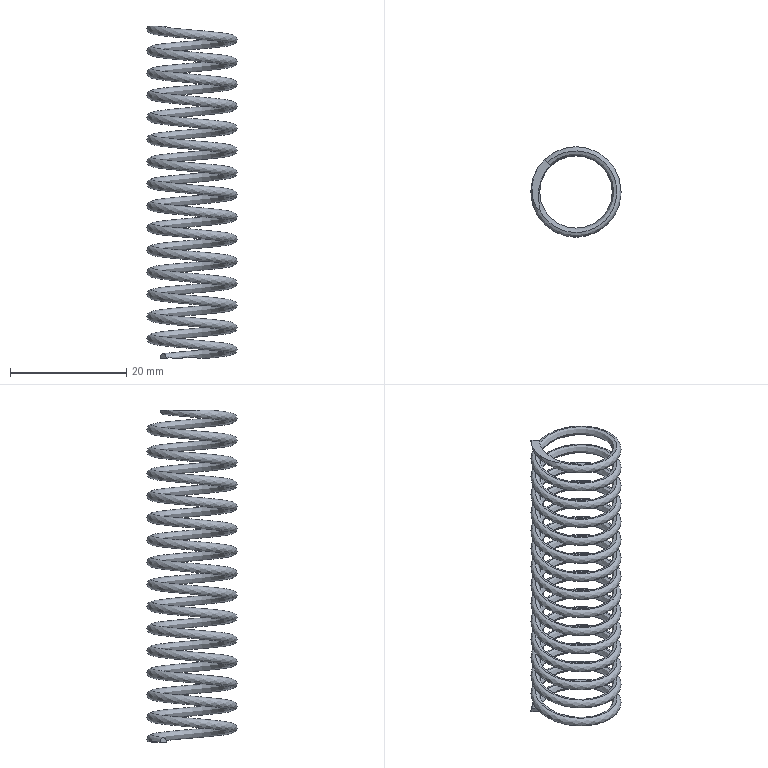Part | STEP file | Spring | 1 solid | 6 faces | box 15.5 x 15.5 x 57 mm | volume 1160 mm3 | plane 4 | spline 2